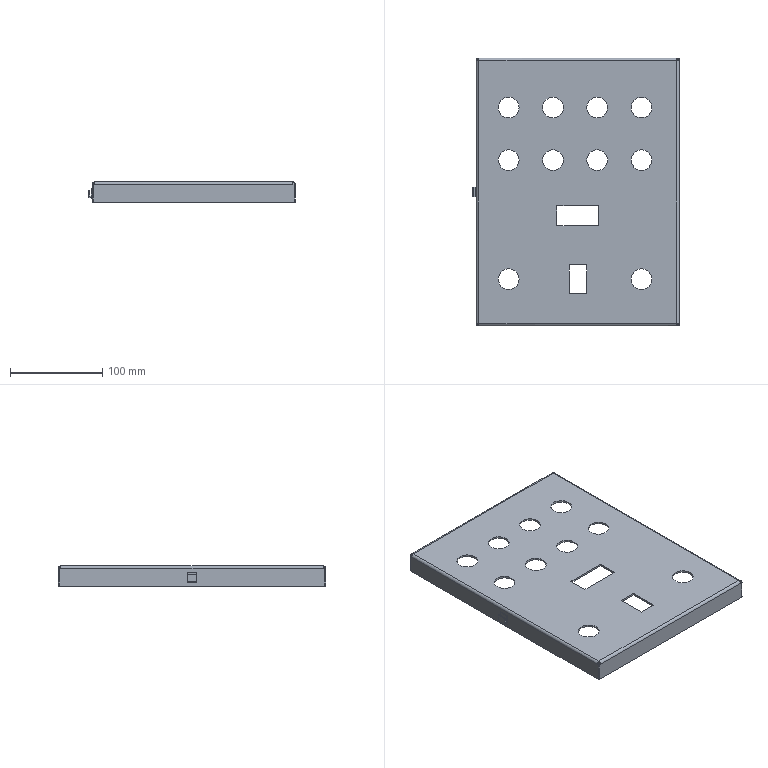Part | STEP file | Upper control box cover | 1 solid | 97 faces | box 224 x 290 x 22 mm | volume 182684 mm3 | plane 41 | cylinder 36 | spline 20 | commonest cylinder face diameters 22.5 x20 1.473 x4 2 x4 5.473 x4 5 x2 10 x2